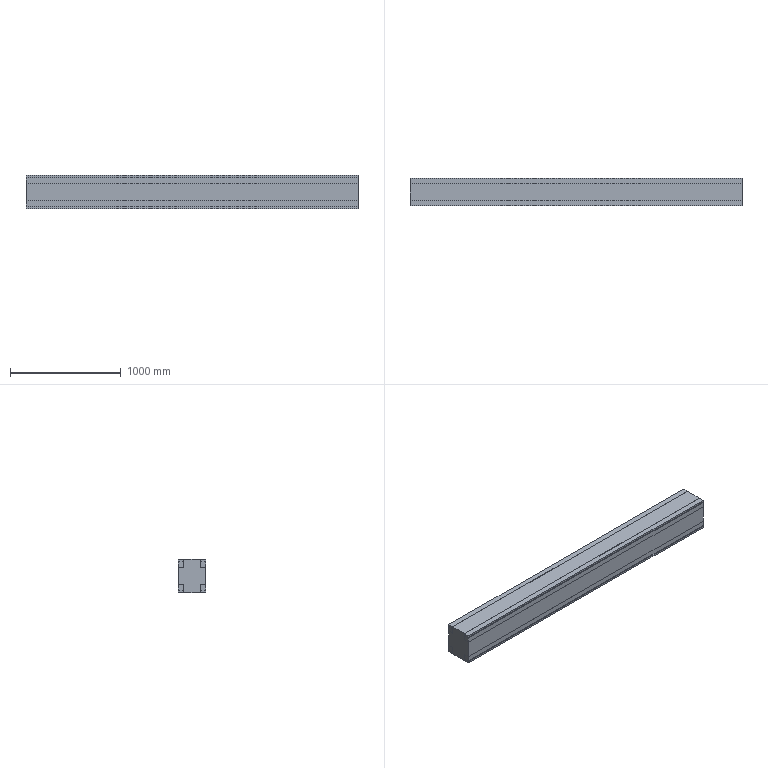Part | SolidWorks | features ICE 2, MirrorSolid 2, Extrusion 1 | 5 solids | 70 faces | box 3000 x 250 x 300 mm | volume 221738400 mm3 | plane 70